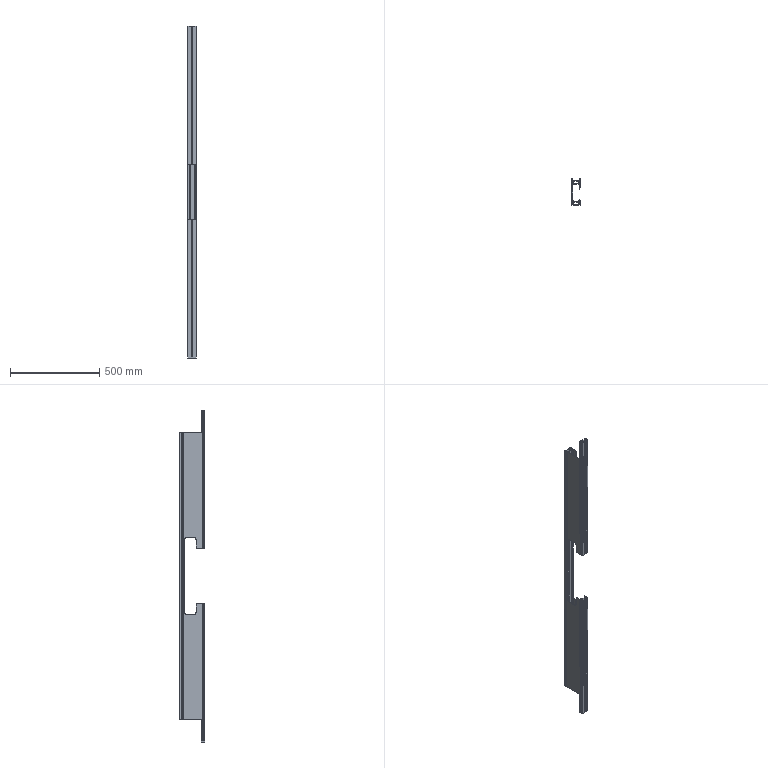Part | SolidWorks | features ICE 11, Fillet 9, MirrorPattern 2, Extrusion 1, LPattern 1 | 1 solid | 198 faces | box 45 x 145 x 1860 mm | volume 1760118 mm3 | plane 181 | cylinder 17 | commonest cylinder face diameters 4 x9 20 x7 3 x1